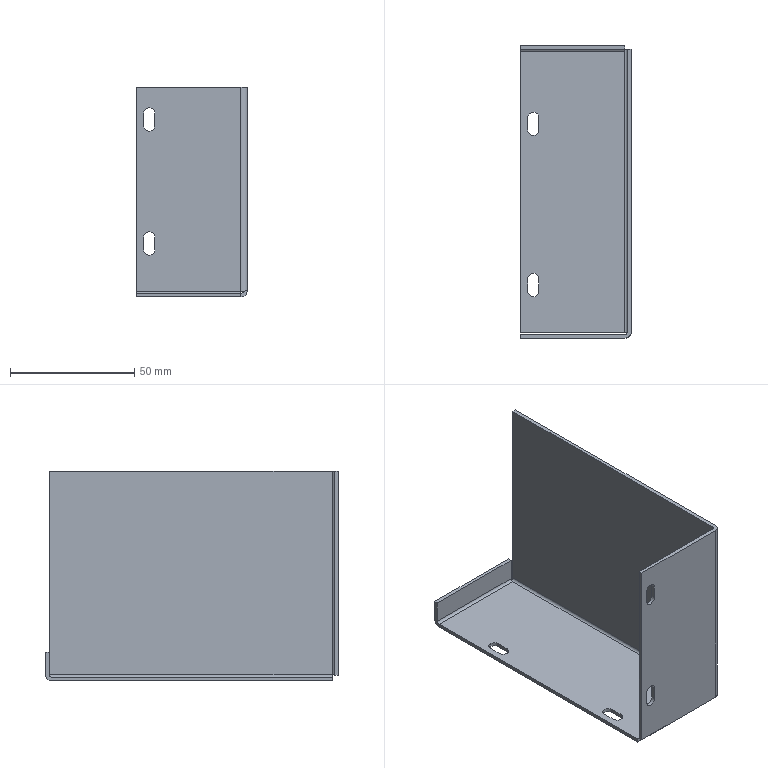Part | SolidWorks | features BaseBody 1 | 1 solid | 41 faces | box 44.5 x 118 x 84.5 mm | volume 27663 mm3 | plane 25 | cylinder 14 | spline 2 | commonest cylinder face diameters 4.5 x8 2 x3 5 x3
STEP:
#1=CARTESIAN_POINT('',(-44.5,115.,10.));
#2=VERTEX_POINT('',#1);
#3=CARTESIAN_POINT('',(-2.5,115.,10.));
#4=VERTEX_POINT('',#3);
#5=CARTESIAN_POINT('',(-2.5,115.,10.));
#6=DIRECTION('',(1.,0.,0.));
#7=VECTOR('',#6,1000.);
#8=LINE('',#5,#7);
#9=EDGE_CURVE('',#2,#4,#8,.T.);
#10=ORIENTED_EDGE('',*,*,#9,.T.);
#11=CARTESIAN_POINT('',(-2.5,116.5,10.));
#12=VERTEX_POINT('',#11);
#13=CARTESIAN_POINT('',(-2.5,116.5,10.));
#14=DIRECTION('',(0.,-1.,0.));
#15=VECTOR('',#14,1000.);
#16=LINE('',#13,#15);
#17=EDGE_CURVE('',#12,#4,#16,.T.);
#18=ORIENTED_EDGE('',*,*,#17,.F.);
#19=CARTESIAN_POINT('',(-44.5,116.5,10.));
#20=VERTEX_POINT('',#19);
#21=CARTESIAN_POINT('',(-2.5,116.5,10.));
#22=DIRECTION('',(1.,0.,0.));
#23=VECTOR('',#22,1000.);
#24=LINE('',#21,#23);
#25=EDGE_CURVE('',#20,#12,#24,.T.);
#26=ORIENTED_EDGE('',*,*,#25,.F.);
#27=CARTESIAN_POINT('',(-44.5,116.5,10.));
#28=DIRECTION('',(0.,-1.,0.));
#29=VECTOR('',#28,1000.);
#30=LINE('',#27,#29);
#31=EDGE_CURVE('',#20,#2,#30,.T.);
#32=ORIENTED_EDGE('',*,*,#31,.T.);
#33=EDGE_LOOP('',(#10,#18,#26,#32));
#34=FACE_OUTER_BOUND('',#33,.T.);
#35=CARTESIAN_POINT('',(-2.5,116.5,10.));
#36=DIRECTION('',(0.,0.,-1.));
#37=DIRECTION('',(0.,-1.,0.));
#38=AXIS2_PLACEMENT_3D('',#35,#36,#37);
#39=PLANE('',#38);
#40=ADVANCED_FACE('',(#34),#39,.F.);
#41=CARTESIAN_POINT('',(-44.5,115.,1.));
#42=VERTEX_POINT('',#41);
#43=CARTESIAN_POINT('',(-44.5,115.,10.));
#44=DIRECTION('',(0.,0.,1.));
#45=VECTOR('',#44,1000.);
#46=LINE('',#43,#45);
#47=EDGE_CURVE('',#42,#2,#46,.T.);
#48=ORIENTED_EDGE('',*,*,#47,.F.);
#49=CARTESIAN_POINT('',(-2.5,115.,1.));
#50=VERTEX_POINT('',#49);
#51=CARTESIAN_POINT('',(-2.5,115.,1.));
#52=DIRECTION('',(-1.,0.,0.));
#53=VECTOR('',#52,1000.);
#54=LINE('',#51,#53);
#55=EDGE_CURVE('',#50,#42,#54,.T.);
#56=ORIENTED_EDGE('',*,*,#55,.F.);
#57=CARTESIAN_POINT('',(-2.5,115.,0.));
#58=DIRECTION('',(0.,0.,-1.));
#59=VECTOR('',#58,1000.);
#60=LINE('',#57,#59);
#61=EDGE_CURVE('',#4,#50,#60,.T.);
#62=ORIENTED_EDGE('',*,*,#61,.F.);
#63=ORIENTED_EDGE('',*,*,#9,.F.);
#64=EDGE_LOOP('',(#48,#56,#62,#63));
#65=FACE_OUTER_BOUND('',#64,.T.);
#66=CARTESIAN_POINT('',(0.,115.,0.));
#67=DIRECTION('',(0.,-1.,0.));
#68=DIRECTION('',(-1.,0.,0.));
#69=AXIS2_PLACEMENT_3D('',#66,#67,#68);
#70=PLANE('',#69);
#71=ADVANCED_FACE('',(#65),#70,.T.);
#72=CARTESIAN_POINT('',(-44.5,116.5,1.));
#73=VERTEX_POINT('',#72);
#74=CARTESIAN_POINT('',(-2.5,116.5,1.));
#75=VERTEX_POINT('',#74);
#76=CARTESIAN_POINT('',(0.,116.5,1.));
#77=DIRECTION('',(1.,0.,0.));
#78=VECTOR('',#77,1000.);
#79=LINE('',#76,#78);
#80=EDGE_CURVE('',#73,#75,#79,.T.);
#81=ORIENTED_EDGE('',*,*,#80,.F.);
#82=CARTESIAN_POINT('',(-44.5,116.5,10.));
#83=DIRECTION('',(0.,0.,1.));
#84=VECTOR('',#83,1000.);
#85=LINE('',#82,#84);
#86=EDGE_CURVE('',#73,#20,#85,.T.);
#87=ORIENTED_EDGE('',*,*,#86,.T.);
#88=ORIENTED_EDGE('',*,*,#25,.T.);
#89=CARTESIAN_POINT('',(-2.5,116.5,0.));
#90=DIRECTION('',(0.,0.,-1.));
#91=VECTOR('',#90,1000.);
#92=LINE('',#89,#91);
#93=EDGE_CURVE('',#12,#75,#92,.T.);
#94=ORIENTED_EDGE('',*,*,#93,.T.);
#95=EDGE_LOOP('',(#81,#87,#88,#94));
#96=FACE_OUTER_BOUND('',#95,.T.);
#97=CARTESIAN_POINT('',(0.,116.5,0.));
#98=DIRECTION('',(0.,-1.,0.));
#99=DIRECTION('',(-1.,0.,0.));
#100=AXIS2_PLACEMENT_3D('',#97,#98,#99);
#101=PLANE('',#100);
#102=ADVANCED_FACE('',(#96),#101,.F.);
#103=CARTESIAN_POINT('',(-44.5,114.,0.));
#104=VERTEX_POINT('',#103);
#105=CARTESIAN_POINT('',(-2.5,114.,0.));
#106=VERTEX_POINT('',#105);
#107=CARTESIAN_POINT('',(-44.5,114.,0.));
#108=DIRECTION('',(1.,0.,0.));
#109=VECTOR('',#108,1000.);
#110=LINE('',#107,#109);
#111=EDGE_CURVE('',#104,#106,#110,.T.);
#112=ORIENTED_EDGE('',*,*,#111,.T.);
#113=CARTESIAN_POINT('',(-2.5,114.,1.));
#114=DIRECTION('',(1.,0.,0.));
#115=DIRECTION('',(0.,0.,1.));
#116=AXIS2_PLACEMENT_3D('',#113,#114,#115);
#117=CIRCLE('',#116,1.);
#118=EDGE_CURVE('',#106,#50,#117,.T.);
#119=ORIENTED_EDGE('',*,*,#118,.T.);
#120=ORIENTED_EDGE('',*,*,#55,.T.);
#121=CARTESIAN_POINT('',(-44.5,114.,1.));
#122=DIRECTION('',(-1.,0.,0.));
#123=DIRECTION('',(0.,0.,1.));
#124=AXIS2_PLACEMENT_3D('',#121,#122,#123);
#125=CIRCLE('',#124,1.);
#126=EDGE_CURVE('',#42,#104,#125,.T.);
#127=ORIENTED_EDGE('',*,*,#126,.T.);
#128=EDGE_LOOP('',(#112,#119,#120,#127));
#129=FACE_OUTER_BOUND('',#128,.T.);
#130=CARTESIAN_POINT('',(-44.5,114.,1.));
#131=DIRECTION('',(-1.,0.,0.));
#132=DIRECTION('',(0.,1.,0.));
#133=AXIS2_PLACEMENT_3D('',#130,#131,#132);
#134=CYLINDRICAL_SURFACE('',#133,1.);
#135=ADVANCED_FACE('',(#129),#134,.F.);
#136=CARTESIAN_POINT('',(-44.5,114.,-1.5));
#137=VERTEX_POINT('',#136);
#138=CARTESIAN_POINT('',(-2.5,114.,-1.5));
#139=VERTEX_POINT('',#138);
#140=CARTESIAN_POINT('',(-44.5,114.,-1.5));
#141=DIRECTION('',(1.,0.,0.));
#142=VECTOR('',#141,1000.);
#143=LINE('',#140,#142);
#144=EDGE_CURVE('',#137,#139,#143,.T.);
#145=ORIENTED_EDGE('',*,*,#144,.F.);
#146=CARTESIAN_POINT('',(-44.5,114.,1.));
#147=DIRECTION('',(-1.,0.,0.));
#148=DIRECTION('',(0.,0.,1.));
#149=AXIS2_PLACEMENT_3D('',#146,#147,#148);
#150=CIRCLE('',#149,2.5);
#151=EDGE_CURVE('',#73,#137,#150,.T.);
#152=ORIENTED_EDGE('',*,*,#151,.F.);
#153=ORIENTED_EDGE('',*,*,#80,.T.);
#154=CARTESIAN_POINT('',(-2.5,115.,-1.291));
#155=VERTEX_POINT('',#154);
#156=CARTESIAN_POINT('',(-2.5,114.,1.));
#157=DIRECTION('',(1.,0.,0.));
#158=DIRECTION('',(0.,0.,1.));
#159=AXIS2_PLACEMENT_3D('',#156,#157,#158);
#160=CIRCLE('',#159,2.5);
#161=EDGE_CURVE('',#155,#75,#160,.T.);
#162=ORIENTED_EDGE('',*,*,#161,.F.);
#163=CARTESIAN_POINT('',(-2.5,114.,1.));
#164=DIRECTION('',(1.,0.,0.));
#165=DIRECTION('',(0.,0.,1.));
#166=AXIS2_PLACEMENT_3D('',#163,#164,#165);
#167=CIRCLE('',#166,2.5);
#168=EDGE_CURVE('',#139,#155,#167,.T.);
#169=ORIENTED_EDGE('',*,*,#168,.F.);
#170=EDGE_LOOP('',(#145,#152,#153,#162,#169));
#171=FACE_OUTER_BOUND('',#170,.T.);
#172=CARTESIAN_POINT('',(-44.5,114.,1.));
#173=DIRECTION('',(-1.,0.,0.));
#174=DIRECTION('',(0.,1.,0.));
#175=AXIS2_PLACEMENT_3D('',#172,#173,#174);
#176=CYLINDRICAL_SURFACE('',#175,2.5);
#177=ADVANCED_FACE('',(#171),#176,.T.);
#178=CARTESIAN_POINT('',(-2.5,115.,0.));
#179=VERTEX_POINT('',#178);
#180=CARTESIAN_POINT('',(-2.5,115.,0.));
#181=DIRECTION('',(0.,-1.,0.));
#182=VECTOR('',#181,1000.);
#183=LINE('',#180,#182);
#184=EDGE_CURVE('',#179,#106,#183,.T.);
#185=ORIENTED_EDGE('',*,*,#184,.F.);
#186=CARTESIAN_POINT('',(-2.5,115.,0.));
#187=DIRECTION('',(0.,0.,-1.));
#188=VECTOR('',#187,1000.);
#189=LINE('',#186,#188);
#190=EDGE_CURVE('',#179,#155,#189,.T.);
#191=ORIENTED_EDGE('',*,*,#190,.T.);
#192=ORIENTED_EDGE('',*,*,#161,.T.);
#193=ORIENTED_EDGE('',*,*,#93,.F.);
#194=ORIENTED_EDGE('',*,*,#17,.T.);
#195=ORIENTED_EDGE('',*,*,#61,.T.);
#196=ORIENTED_EDGE('',*,*,#118,.F.);
#197=EDGE_LOOP('',(#185,#191,#192,#193,#194,#195,#196));
#198=FACE_OUTER_BOUND('',#197,.T.);
#199=CARTESIAN_POINT('',(-2.5,114.,1.));
#200=DIRECTION('',(1.,0.,0.));
#201=DIRECTION('',(0.,0.,1.));
#202=AXIS2_PLACEMENT_3D('',#199,#200,#201);
#203=PLANE('',#202);
#204=ADVANCED_FACE('',(#198),#203,.T.);
#205=CARTESIAN_POINT('',(-41.75,0.,72.5));
#206=VERTEX_POINT('',#205);
#207=CARTESIAN_POINT('',(-41.75,-1.5,72.5));
#208=VERTEX_POINT('',#207);
#209=CARTESIAN_POINT('',(-41.75,115.001,72.5));
#210=DIRECTION('',(0.,-1.,0.));
#211=VECTOR('',#210,1000.);
#212=LINE('',#209,#211);
#213=EDGE_CURVE('',#206,#208,#212,.T.);
#214=ORIENTED_EDGE('',*,*,#213,.T.);
#215=CARTESIAN_POINT('',(-41.75,-1.5,67.5));
#216=VERTEX_POINT('',#215);
#217=CARTESIAN_POINT('',(-41.75,-1.5,72.5));
#218=DIRECTION('',(0.,0.,-1.));
#219=VECTOR('',#218,1000.);
#220=LINE('',#217,#219);
#221=EDGE_CURVE('',#208,#216,#220,.T.);
#222=ORIENTED_EDGE('',*,*,#221,.T.);
#223=CARTESIAN_POINT('',(-41.75,0.,67.5));
#224=VERTEX_POINT('',#223);
#225=CARTESIAN_POINT('',(-41.75,115.001,67.5));
#226=DIRECTION('',(0.,-1.,0.));
#227=VECTOR('',#226,1000.);
#228=LINE('',#225,#227);
#229=EDGE_CURVE('',#224,#216,#228,.T.);
#230=ORIENTED_EDGE('',*,*,#229,.F.);
#231=CARTESIAN_POINT('',(-41.75,0.,72.5));
#232=DIRECTION('',(0.,0.,-1.));
#233=VECTOR('',#232,1000.);
#234=LINE('',#231,#233);
#235=EDGE_CURVE('',#206,#224,#234,.T.);
#236=ORIENTED_EDGE('',*,*,#235,.F.);
#237=EDGE_LOOP('',(#214,#222,#230,#236));
#238=FACE_OUTER_BOUND('',#237,.T.);
#239=CARTESIAN_POINT('',(-41.75,115.001,72.5));
#240=DIRECTION('',(-1.,0.,0.));
#241=DIRECTION('',(0.,1.,0.));
#242=AXIS2_PLACEMENT_3D('',#239,#240,#241);
#243=PLANE('',#242);
#244=ADVANCED_FACE('',(#238),#243,.F.);
#245=ORIENTED_EDGE('',*,*,#229,.T.);
#246=CARTESIAN_POINT('',(-37.25,-1.5,67.5));
#247=VERTEX_POINT('',#246);
#248=CARTESIAN_POINT('',(-39.5,-1.5,67.5));
#249=DIRECTION('',(0.,-1.,0.));
#250=DIRECTION('',(-1.,0.,0.));
#251=AXIS2_PLACEMENT_3D('',#248,#249,#250);
#252=CIRCLE('',#251,2.25);
#253=EDGE_CURVE('',#216,#247,#252,.T.);
#254=ORIENTED_EDGE('',*,*,#253,.T.);
#255=CARTESIAN_POINT('',(-37.25,0.,67.5));
#256=VERTEX_POINT('',#255);
#257=CARTESIAN_POINT('',(-37.25,115.001,67.5));
#258=DIRECTION('',(0.,-1.,0.));
#259=VECTOR('',#258,1000.);
#260=LINE('',#257,#259);
#261=EDGE_CURVE('',#256,#247,#260,.T.);
#262=ORIENTED_EDGE('',*,*,#261,.F.);
#263=CARTESIAN_POINT('',(-39.5,0.,67.5));
#264=DIRECTION('',(0.,-1.,0.));
#265=DIRECTION('',(-1.,0.,0.));
#266=AXIS2_PLACEMENT_3D('',#263,#264,#265);
#267=CIRCLE('',#266,2.25);
#268=EDGE_CURVE('',#224,#256,#267,.T.);
#269=ORIENTED_EDGE('',*,*,#268,.F.);
#270=EDGE_LOOP('',(#245,#254,#262,#269));
#271=FACE_OUTER_BOUND('',#270,.T.);
#272=CARTESIAN_POINT('',(-39.5,115.001,67.5));
#273=DIRECTION('',(0.,-1.,0.));
#274=DIRECTION('',(1.,0.,0.));
#275=AXIS2_PLACEMENT_3D('',#272,#273,#274);
#276=CYLINDRICAL_SURFACE('',#275,2.25);
#277=ADVANCED_FACE('',(#271),#276,.F.);
#278=ORIENTED_EDGE('',*,*,#261,.T.);
#279=CARTESIAN_POINT('',(-37.25,-1.5,72.5));
#280=VERTEX_POINT('',#279);
#281=CARTESIAN_POINT('',(-37.25,-1.5,72.5));
#282=DIRECTION('',(0.,0.,1.));
#283=VECTOR('',#282,1000.);
#284=LINE('',#281,#283);
#285=EDGE_CURVE('',#247,#280,#284,.T.);
#286=ORIENTED_EDGE('',*,*,#285,.T.);
#287=CARTESIAN_POINT('',(-37.25,0.,72.5));
#288=VERTEX_POINT('',#287);
#289=CARTESIAN_POINT('',(-37.25,115.001,72.5));
#290=DIRECTION('',(0.,-1.,0.));
#291=VECTOR('',#290,1000.);
#292=LINE('',#289,#291);
#293=EDGE_CURVE('',#288,#280,#292,.T.);
#294=ORIENTED_EDGE('',*,*,#293,.F.);
#295=CARTESIAN_POINT('',(-37.25,0.,72.5));
#296=DIRECTION('',(0.,0.,1.));
#297=VECTOR('',#296,1000.);
#298=LINE('',#295,#297);
#299=EDGE_CURVE('',#256,#288,#298,.T.);
#300=ORIENTED_EDGE('',*,*,#299,.F.);
#301=EDGE_LOOP('',(#278,#286,#294,#300));
#302=FACE_OUTER_BOUND('',#301,.T.);
#303=CARTESIAN_POINT('',(-37.25,115.001,72.5));
#304=DIRECTION('',(1.,0.,0.));
#305=DIRECTION('',(0.,1.,0.));
#306=AXIS2_PLACEMENT_3D('',#303,#304,#305);
#307=PLANE('',#306);
#308=ADVANCED_FACE('',(#302),#307,.F.);
#309=ORIENTED_EDGE('',*,*,#293,.T.);
#310=CARTESIAN_POINT('',(-39.5,-1.5,72.5));
#311=DIRECTION('',(0.,-1.,0.));
#312=DIRECTION('',(-1.,0.,0.));
#313=AXIS2_PLACEMENT_3D('',#310,#311,#312);
#314=CIRCLE('',#313,2.25);
#315=EDGE_CURVE('',#280,#208,#314,.T.);
#316=ORIENTED_EDGE('',*,*,#315,.T.);
#317=ORIENTED_EDGE('',*,*,#213,.F.);
#318=CARTESIAN_POINT('',(-39.5,0.,72.5));
#319=DIRECTION('',(0.,-1.,0.));
#320=DIRECTION('',(-1.,0.,0.));
#321=AXIS2_PLACEMENT_3D('',#318,#319,#320);
#322=CIRCLE('',#321,2.25);
#323=EDGE_CURVE('',#288,#206,#322,.T.);
#324=ORIENTED_EDGE('',*,*,#323,.F.);
#325=EDGE_LOOP('',(#309,#316,#317,#324));
#326=FACE_OUTER_BOUND('',#325,.T.);
#327=CARTESIAN_POINT('',(-39.5,115.001,72.5));
#328=DIRECTION('',(0.,-1.,0.));
#329=DIRECTION('',(1.,0.,0.));
#330=AXIS2_PLACEMENT_3D('',#327,#328,#329);
#331=CYLINDRICAL_SURFACE('',#330,2.25);
#332=ADVANCED_FACE('',(#326),#331,.F.);
#333=CARTESIAN_POINT('',(-37.25,0.,17.5));
#334=VERTEX_POINT('',#333);
#335=CARTESIAN_POINT('',(-37.25,-1.5,17.5));
#336=VERTEX_POINT('',#335);
#337=CARTESIAN_POINT('',(-37.25,115.001,17.5));
#338=DIRECTION('',(0.,-1.,0.));
#339=VECTOR('',#338,1000.);
#340=LINE('',#337,#339);
#341=EDGE_CURVE('',#334,#336,#340,.T.);
#342=ORIENTED_EDGE('',*,*,#341,.T.);
#343=CARTESIAN_POINT('',(-37.25,-1.5,22.5));
#344=VERTEX_POINT('',#343);
#345=CARTESIAN_POINT('',(-37.25,-1.5,17.5));
#346=DIRECTION('',(0.,0.,1.));
#347=VECTOR('',#346,1000.);
#348=LINE('',#345,#347);
#349=EDGE_CURVE('',#336,#344,#348,.T.);
#350=ORIENTED_EDGE('',*,*,#349,.T.);
#351=CARTESIAN_POINT('',(-37.25,0.,22.5));
#352=VERTEX_POINT('',#351);
#353=CARTESIAN_POINT('',(-37.25,115.001,22.5));
#354=DIRECTION('',(0.,-1.,0.));
#355=VECTOR('',#354,1000.);
#356=LINE('',#353,#355);
#357=EDGE_CURVE('',#352,#344,#356,.T.);
#358=ORIENTED_EDGE('',*,*,#357,.F.);
#359=CARTESIAN_POINT('',(-37.25,0.,17.5));
#360=DIRECTION('',(0.,0.,1.));
#361=VECTOR('',#360,1000.);
#362=LINE('',#359,#361);
#363=EDGE_CURVE('',#334,#352,#362,.T.);
#364=ORIENTED_EDGE('',*,*,#363,.F.);
#365=EDGE_LOOP('',(#342,#350,#358,#364));
#366=FACE_OUTER_BOUND('',#365,.T.);
#367=CARTESIAN_POINT('',(-37.25,115.001,17.5));
#368=DIRECTION('',(1.,0.,0.));
#369=DIRECTION('',(0.,1.,0.));
#370=AXIS2_PLACEMENT_3D('',#367,#368,#369);
#371=PLANE('',#370);
#372=ADVANCED_FACE('',(#366),#371,.F.);
#373=ORIENTED_EDGE('',*,*,#357,.T.);
#374=CARTESIAN_POINT('',(-41.75,-1.5,22.5));
#375=VERTEX_POINT('',#374);
#376=CARTESIAN_POINT('',(-39.5,-1.5,22.5));
#377=DIRECTION('',(0.,-1.,0.));
#378=DIRECTION('',(1.,0.,0.));
#379=AXIS2_PLACEMENT_3D('',#376,#377,#378);
#380=CIRCLE('',#379,2.25);
#381=EDGE_CURVE('',#344,#375,#380,.T.);
#382=ORIENTED_EDGE('',*,*,#381,.T.);
#383=CARTESIAN_POINT('',(-41.75,0.,22.5));
#384=VERTEX_POINT('',#383);
#385=CARTESIAN_POINT('',(-41.75,115.001,22.5));
#386=DIRECTION('',(0.,-1.,0.));
#387=VECTOR('',#386,1000.);
#388=LINE('',#385,#387);
#389=EDGE_CURVE('',#384,#375,#388,.T.);
#390=ORIENTED_EDGE('',*,*,#389,.F.);
#391=CARTESIAN_POINT('',(-39.5,0.,22.5));
#392=DIRECTION('',(0.,-1.,0.));
#393=DIRECTION('',(-1.,0.,0.));
#394=AXIS2_PLACEMENT_3D('',#391,#392,#393);
#395=CIRCLE('',#394,2.25);
#396=EDGE_CURVE('',#352,#384,#395,.T.);
#397=ORIENTED_EDGE('',*,*,#396,.F.);
#398=EDGE_LOOP('',(#373,#382,#390,#397));
#399=FACE_OUTER_BOUND('',#398,.T.);
#400=CARTESIAN_POINT('',(-39.5,115.001,22.5));
#401=DIRECTION('',(0.,-1.,0.));
#402=DIRECTION('',(1.,0.,0.));
#403=AXIS2_PLACEMENT_3D('',#400,#401,#402);
#404=CYLINDRICAL_SURFACE('',#403,2.25);
#405=ADVANCED_FACE('',(#399),#404,.F.);
#406=ORIENTED_EDGE('',*,*,#389,.T.);
#407=CARTESIAN_POINT('',(-41.75,-1.5,17.5));
#408=VERTEX_POINT('',#407);
#409=CARTESIAN_POINT('',(-41.75,-1.5,17.5));
#410=DIRECTION('',(0.,0.,-1.));
#411=VECTOR('',#410,1000.);
#412=LINE('',#409,#411);
#413=EDGE_CURVE('',#375,#408,#412,.T.);
#414=ORIENTED_EDGE('',*,*,#413,.T.);
#415=CARTESIAN_POINT('',(-41.75,0.,17.5));
#416=VERTEX_POINT('',#415);
#417=CARTESIAN_POINT('',(-41.75,115.001,17.5));
#418=DIRECTION('',(0.,-1.,0.));
#419=VECTOR('',#418,1000.);
#420=LINE('',#417,#419);
#421=EDGE_CURVE('',#416,#408,#420,.T.);
#422=ORIENTED_EDGE('',*,*,#421,.F.);
#423=CARTESIAN_POINT('',(-41.75,0.,17.5));
#424=DIRECTION('',(0.,0.,-1.));
#425=VECTOR('',#424,1000.);
#426=LINE('',#423,#425);
#427=EDGE_CURVE('',#384,#416,#426,.T.);
#428=ORIENTED_EDGE('',*,*,#427,.F.);
#429=EDGE_LOOP('',(#406,#414,#422,#428));
#430=FACE_OUTER_BOUND('',#429,.T.);
#431=CARTESIAN_POINT('',(-41.75,115.001,17.5));
#432=DIRECTION('',(-1.,0.,0.));
#433=DIRECTION('',(0.,1.,0.));
#434=AXIS2_PLACEMENT_3D('',#431,#432,#433);
#435=PLANE('',#434);
#436=ADVANCED_FACE('',(#430),#435,.F.);
#437=ORIENTED_EDGE('',*,*,#421,.T.);
#438=CARTESIAN_POINT('',(-39.5,-1.5,17.5));
#439=DIRECTION('',(0.,-1.,0.));
#440=DIRECTION('',(1.,0.,0.));
#441=AXIS2_PLACEMENT_3D('',#438,#439,#440);
#442=CIRCLE('',#441,2.25);
#443=EDGE_CURVE('',#408,#336,#442,.T.);
#444=ORIENTED_EDGE('',*,*,#443,.T.);
#445=ORIENTED_EDGE('',*,*,#341,.F.);
#446=CARTESIAN_POINT('',(-39.5,0.,17.5));
#447=DIRECTION('',(0.,-1.,0.));
#448=DIRECTION('',(-1.,0.,0.));
#449=AXIS2_PLACEMENT_3D('',#446,#447,#448);
#450=CIRCLE('',#449,2.25);
#451=EDGE_CURVE('',#416,#334,#450,.T.);
#452=ORIENTED_EDGE('',*,*,#451,.F.);
#453=EDGE_LOOP('',(#437,#444,#445,#452));
#454=FACE_OUTER_BOUND('',#453,.T.);
#455=CARTESIAN_POINT('',(-39.5,115.001,17.5));
#456=DIRECTION('',(0.,-1.,0.));
#457=DIRECTION('',(1.,0.,0.));
#458=AXIS2_PLACEMENT_3D('',#455,#456,#457);
#459=CYLINDRICAL_SURFACE('',#458,2.25);
#460=ADVANCED_FACE('',(#454),#459,.F.);
#461=CARTESIAN_POINT('',(-41.75,22.5,0.));
#462=VERTEX_POINT('',#461);
#463=CARTESIAN_POINT('',(-41.75,17.5,0.));
#464=VERTEX_POINT('',#463);
#465=CARTESIAN_POINT('',(-41.75,17.5,0.));
#466=DIRECTION('',(0.,-1.,0.));
#467=VECTOR('',#466,1000.);
#468=LINE('',#465,#467);
#469=EDGE_CURVE('',#462,#464,#468,.T.);
#470=ORIENTED_EDGE('',*,*,#469,.T.);
#471=CARTESIAN_POINT('',(-41.75,17.5,-1.5));
#472=VERTEX_POINT('',#471);
#473=CARTESIAN_POINT('',(-41.75,17.5,83.001));
#474=DIRECTION('',(0.,0.,-1.));
#475=VECTOR('',#474,1000.);
#476=LINE('',#473,#475);
#477=EDGE_CURVE('',#464,#472,#476,.T.);
#478=ORIENTED_EDGE('',*,*,#477,.T.);
#479=CARTESIAN_POINT('',(-41.75,22.5,-1.5));
#480=VERTEX_POINT('',#479);
#481=CARTESIAN_POINT('',(-41.75,17.5,-1.5));
#482=DIRECTION('',(0.,1.,0.));
#483=VECTOR('',#482,1000.);
#484=LINE('',#481,#483);
#485=EDGE_CURVE('',#472,#480,#484,.T.);
#486=ORIENTED_EDGE('',*,*,#485,.T.);
#487=CARTESIAN_POINT('',(-41.75,22.5,83.001));
#488=DIRECTION('',(0.,0.,-1.));
#489=VECTOR('',#488,1000.);
#490=LINE('',#487,#489);
#491=EDGE_CURVE('',#462,#480,#490,.T.);
#492=ORIENTED_EDGE('',*,*,#491,.F.);
#493=EDGE_LOOP('',(#470,#478,#486,#492));
#494=FACE_OUTER_BOUND('',#493,.T.);
#495=CARTESIAN_POINT('',(-41.75,17.5,83.001));
#496=DIRECTION('',(-1.,0.,0.));
#497=DIRECTION('',(0.,0.,1.));
#498=AXIS2_PLACEMENT_3D('',#495,#496,#497);
#499=PLANE('',#498);
#500=ADVANCED_FACE('',(#494),#499,.F.);
#501=CARTESIAN_POINT('',(-37.25,22.5,0.));
#502=VERTEX_POINT('',#501);
#503=CARTESIAN_POINT('',(-39.5,22.5,0.));
#504=DIRECTION('',(0.,0.,1.));
#505=DIRECTION('',(-1.,0.,0.));
#506=AXIS2_PLACEMENT_3D('',#503,#504,#505);
#507=CIRCLE('',#506,2.25);
#508=EDGE_CURVE('',#502,#462,#507,.T.);
#509=ORIENTED_EDGE('',*,*,#508,.T.);
#510=ORIENTED_EDGE('',*,*,#491,.T.);
#511=CARTESIAN_POINT('',(-37.25,22.5,-1.5));
#512=VERTEX_POINT('',#511);
#513=CARTESIAN_POINT('',(-39.5,22.5,-1.5));
#514=DIRECTION('',(0.,0.,-1.));
#515=DIRECTION('',(1.,0.,0.));
#516=AXIS2_PLACEMENT_3D('',#513,#514,#515);
#517=CIRCLE('',#516,2.25);
#518=EDGE_CURVE('',#480,#512,#517,.T.);
#519=ORIENTED_EDGE('',*,*,#518,.T.);
#520=CARTESIAN_POINT('',(-37.25,22.5,83.001));
#521=DIRECTION('',(0.,0.,-1.));
#522=VECTOR('',#521,1000.);
#523=LINE('',#520,#522);
#524=EDGE_CURVE('',#502,#512,#523,.T.);
#525=ORIENTED_EDGE('',*,*,#524,.F.);
#526=EDGE_LOOP('',(#509,#510,#519,#525));
#527=FACE_OUTER_BOUND('',#526,.T.);
#528=CARTESIAN_POINT('',(-39.5,22.5,83.001));
#529=DIRECTION('',(0.,0.,-1.));
#530=DIRECTION('',(-1.,0.,0.));
#531=AXIS2_PLACEMENT_3D('',#528,#529,#530);
#532=CYLINDRICAL_SURFACE('',#531,2.25);
#533=ADVANCED_FACE('',(#527),#532,.F.);
#534=CARTESIAN_POINT('',(-37.25,17.5,0.));
#535=VERTEX_POINT('',#534);
#536=CARTESIAN_POINT('',(-37.25,17.5,0.));
#537=DIRECTION('',(0.,1.,0.));
#538=VECTOR('',#537,1000.);
#539=LINE('',#536,#538);
#540=EDGE_CURVE('',#535,#502,#539,.T.);
#541=ORIENTED_EDGE('',*,*,#540,.T.);
#542=ORIENTED_EDGE('',*,*,#524,.T.);
#543=CARTESIAN_POINT('',(-37.25,17.5,-1.5));
#544=VERTEX_POINT('',#543);
#545=CARTESIAN_POINT('',(-37.25,17.5,-1.5));
#546=DIRECTION('',(0.,-1.,0.));
#547=VECTOR('',#546,1000.);
#548=LINE('',#545,#547);
#549=EDGE_CURVE('',#512,#544,#548,.T.);
#550=ORIENTED_EDGE('',*,*,#549,.T.);
#551=CARTESIAN_POINT('',(-37.25,17.5,83.001));
#552=DIRECTION('',(0.,0.,-1.));
#553=VECTOR('',#552,1000.);
#554=LINE('',#551,#553);
#555=EDGE_CURVE('',#535,#544,#554,.T.);
#556=ORIENTED_EDGE('',*,*,#555,.F.);
#557=EDGE_LOOP('',(#541,#542,#550,#556));
#558=FACE_OUTER_BOUND('',#557,.T.);
#559=CARTESIAN_POINT('',(-37.25,17.5,83.001));
#560=DIRECTION('',(1.,0.,0.));
#561=DIRECTION('',(0.,0.,1.));
#562=AXIS2_PLACEMENT_3D('',#559,#560,#561);
#563=PLANE('',#562);
#564=ADVANCED_FACE('',(#558),#563,.F.);
#565=CARTESIAN_POINT('',(-39.5,17.5,0.));
#566=DIRECTION('',(0.,0.,1.));
#567=DIRECTION('',(-1.,0.,0.));
#568=AXIS2_PLACEMENT_3D('',#565,#566,#567);
#569=CIRCLE('',#568,2.25);
#570=EDGE_CURVE('',#464,#535,#569,.T.);
#571=ORIENTED_EDGE('',*,*,#570,.T.);
#572=ORIENTED_EDGE('',*,*,#555,.T.);
#573=CARTESIAN_POINT('',(-39.5,17.5,-1.5));
#574=DIRECTION('',(0.,0.,-1.));
#575=DIRECTION('',(1.,0.,0.));
#576=AXIS2_PLACEMENT_3D('',#573,#574,#575);
#577=CIRCLE('',#576,2.25);
#578=EDGE_CURVE('',#544,#472,#577,.T.);
#579=ORIENTED_EDGE('',*,*,#578,.T.);
#580=ORIENTED_EDGE('',*,*,#477,.F.);
#581=EDGE_LOOP('',(#571,#572,#579,#580));
#582=FACE_OUTER_BOUND('',#581,.T.);
#583=CARTESIAN_POINT('',(-39.5,17.5,83.001));
#584=DIRECTION('',(0.,0.,-1.));
#585=DIRECTION('',(-1.,0.,0.));
#586=AXIS2_PLACEMENT_3D('',#583,#584,#585);
#587=CYLINDRICAL_SURFACE('',#586,2.25);
#588=ADVANCED_FACE('',(#582),#587,.F.);
#589=CARTESIAN_POINT('',(-37.25,82.5,0.));
#590=VERTEX_POINT('',#589);
#591=CARTESIAN_POINT('',(-37.25,87.5,0.));
#592=VERTEX_POINT('',#591);
#593=CARTESIAN_POINT('',(-37.25,87.5,0.));
#594=DIRECTION('',(0.,1.,0.));
#595=VECTOR('',#594,1000.);
#596=LINE('',#593,#595);
#597=EDGE_CURVE('',#590,#592,#596,.T.);
#598=ORIENTED_EDGE('',*,*,#597,.T.);
#599=CARTESIAN_POINT('',(-37.25,87.5,-1.5));
#600=VERTEX_POINT('',#599);
#601=CARTESIAN_POINT('',(-37.25,87.5,83.001));
#602=DIRECTION('',(0.,0.,-1.));
#603=VECTOR('',#602,1000.);
#604=LINE('',#601,#603);
#605=EDGE_CURVE('',#592,#600,#604,.T.);
#606=ORIENTED_EDGE('',*,*,#605,.T.);
#607=CARTESIAN_POINT('',(-37.25,82.5,-1.5));
#608=VERTEX_POINT('',#607);
#609=CARTESIAN_POINT('',(-37.25,87.5,-1.5));
#610=DIRECTION('',(0.,-1.,0.));
#611=VECTOR('',#610,1000.);
#612=LINE('',#609,#611);
#613=EDGE_CURVE('',#600,#608,#612,.T.);
#614=ORIENTED_EDGE('',*,*,#613,.T.);
#615=CARTESIAN_POINT('',(-37.25,82.5,83.001));
#616=DIRECTION('',(0.,0.,-1.));
#617=VECTOR('',#616,1000.);
#618=LINE('',#615,#617);
#619=EDGE_CURVE('',#590,#608,#618,.T.);
#620=ORIENTED_EDGE('',*,*,#619,.F.);
#621=EDGE_LOOP('',(#598,#606,#614,#620));
#622=FACE_OUTER_BOUND('',#621,.T.);
#623=CARTESIAN_POINT('',(-37.25,87.5,83.001));
#624=DIRECTION('',(1.,0.,0.));
#625=DIRECTION('',(0.,0.,1.));
#626=AXIS2_PLACEMENT_3D('',#623,#624,#625);
#627=PLANE('',#626);
#628=ADVANCED_FACE('',(#622),#627,.F.);
#629=CARTESIAN_POINT('',(-41.75,82.5,0.));
#630=VERTEX_POINT('',#629);
#631=CARTESIAN_POINT('',(-39.5,82.5,0.));
#632=DIRECTION('',(0.,0.,1.));
#633=DIRECTION('',(-1.,0.,0.));
#634=AXIS2_PLACEMENT_3D('',#631,#632,#633);
#635=CIRCLE('',#634,2.25);
#636=EDGE_CURVE('',#630,#590,#635,.T.);
#637=ORIENTED_EDGE('',*,*,#636,.T.);
#638=ORIENTED_EDGE('',*,*,#619,.T.);
#639=CARTESIAN_POINT('',(-41.75,82.5,-1.5));
#640=VERTEX_POINT('',#639);
#641=CARTESIAN_POINT('',(-39.5,82.5,-1.5));
#642=DIRECTION('',(0.,0.,-1.));
#643=DIRECTION('',(-1.,0.,0.));
#644=AXIS2_PLACEMENT_3D('',#641,#642,#643);
#645=CIRCLE('',#644,2.25);
#646=EDGE_CURVE('',#608,#640,#645,.T.);
#647=ORIENTED_EDGE('',*,*,#646,.T.);
#648=CARTESIAN_POINT('',(-41.75,82.5,83.001));
#649=DIRECTION('',(0.,0.,-1.));
#650=VECTOR('',#649,1000.);
#651=LINE('',#648,#650);
#652=EDGE_CURVE('',#630,#640,#651,.T.);
#653=ORIENTED_EDGE('',*,*,#652,.F.);
#654=EDGE_LOOP('',(#637,#638,#647,#653));
#655=FACE_OUTER_BOUND('',#654,.T.);
#656=CARTESIAN_POINT('',(-39.5,82.5,83.001));
#657=DIRECTION('',(0.,0.,-1.));
#658=DIRECTION('',(-1.,0.,0.));
#659=AXIS2_PLACEMENT_3D('',#656,#657,#658);
#660=CYLINDRICAL_SURFACE('',#659,2.25);
#661=ADVANCED_FACE('',(#655),#660,.F.);
#662=CARTESIAN_POINT('',(-41.75,87.5,0.));
#663=VERTEX_POINT('',#662);
#664=CARTESIAN_POINT('',(-41.75,87.5,0.));
#665=DIRECTION('',(0.,-1.,0.));
#666=VECTOR('',#665,1000.);
#667=LINE('',#664,#666);
#668=EDGE_CURVE('',#663,#630,#667,.T.);
#669=ORIENTED_EDGE('',*,*,#668,.T.);
#670=ORIENTED_EDGE('',*,*,#652,.T.);
#671=CARTESIAN_POINT('',(-41.75,87.5,-1.5));
#672=VERTEX_POINT('',#671);
#673=CARTESIAN_POINT('',(-41.75,87.5,-1.5));
#674=DIRECTION('',(0.,1.,0.));
#675=VECTOR('',#674,1000.);
#676=LINE('',#673,#675);
#677=EDGE_CURVE('',#640,#672,#676,.T.);
#678=ORIENTED_EDGE('',*,*,#677,.T.);
#679=CARTESIAN_POINT('',(-41.75,87.5,83.001));
#680=DIRECTION('',(0.,0.,-1.));
#681=VECTOR('',#680,1000.);
#682=LINE('',#679,#681);
#683=EDGE_CURVE('',#663,#672,#682,.T.);
#684=ORIENTED_EDGE('',*,*,#683,.F.);
#685=EDGE_LOOP('',(#669,#670,#678,#684));
#686=FACE_OUTER_BOUND('',#685,.T.);
#687=CARTESIAN_POINT('',(-41.75,87.5,83.001));
#688=DIRECTION('',(-1.,0.,0.));
#689=DIRECTION('',(0.,0.,1.));
#690=AXIS2_PLACEMENT_3D('',#687,#688,#689);
#691=PLANE('',#690);
#692=ADVANCED_FACE('',(#686),#691,.F.);
#693=CARTESIAN_POINT('',(-39.5,87.5,0.));
#694=DIRECTION('',(0.,0.,1.));
#695=DIRECTION('',(-1.,0.,0.));
#696=AXIS2_PLACEMENT_3D('',#693,#694,#695);
#697=CIRCLE('',#696,2.25);
#698=EDGE_CURVE('',#592,#663,#697,.T.);
#699=ORIENTED_EDGE('',*,*,#698,.T.);
#700=ORIENTED_EDGE('',*,*,#683,.T.);
#701=CARTESIAN_POINT('',(-39.5,87.5,-1.5));
#702=DIRECTION('',(0.,0.,-1.));
#703=DIRECTION('',(-1.,0.,0.));
#704=AXIS2_PLACEMENT_3D('',#701,#702,#703);
#705=CIRCLE('',#704,2.25);
#706=EDGE_CURVE('',#672,#600,#705,.T.);
#707=ORIENTED_EDGE('',*,*,#706,.T.);
#708=ORIENTED_EDGE('',*,*,#605,.F.);
#709=EDGE_LOOP('',(#699,#700,#707,#708));
#710=FACE_OUTER_BOUND('',#709,.T.);
#711=CARTESIAN_POINT('',(-39.5,87.5,83.001));
#712=DIRECTION('',(0.,0.,-1.));
#713=DIRECTION('',(-1.,0.,0.));
#714=AXIS2_PLACEMENT_3D('',#711,#712,#713);
#715=CYLINDRICAL_SURFACE('',#714,2.25);
#716=ADVANCED_FACE('',(#710),#715,.F.);
#717=CARTESIAN_POINT('',(-44.5,0.,0.7071));
#718=VERTEX_POINT('',#717);
#719=CARTESIAN_POINT('',(-44.5,0.,83.));
#720=VERTEX_POINT('',#719);
#721=CARTESIAN_POINT('',(-44.5,0.,0.));
#722=DIRECTION('',(0.,0.,1.));
#723=VECTOR('',#722,1000.);
#724=LINE('',#721,#723);
#725=EDGE_CURVE('',#718,#720,#724,.T.);
#726=ORIENTED_EDGE('',*,*,#725,.F.);
#727=CARTESIAN_POINT('',(-44.5,-1.5,0.7071));
#728=VERTEX_POINT('',#727);
#729=CARTESIAN_POINT('',(-44.5,-1.5,0.7071));
#730=DIRECTION('',(0.,-1.,0.));
#731=VECTOR('',#730,1000.);
#732=LINE('',#729,#731);
#733=EDGE_CURVE('',#718,#728,#732,.T.);
#734=ORIENTED_EDGE('',*,*,#733,.T.);
#735=CARTESIAN_POINT('',(-44.5,-1.5,83.));
#736=VERTEX_POINT('',#735);
#737=CARTESIAN_POINT('',(-44.5,-1.5,0.));
#738=DIRECTION('',(0.,0.,1.));
#739=VECTOR('',#738,1000.);
#740=LINE('',#737,#739);
#741=EDGE_CURVE('',#728,#736,#740,.T.);
#742=ORIENTED_EDGE('',*,*,#741,.T.);
#743=CARTESIAN_POINT('',(-44.5,-1.5,83.));
#744=DIRECTION('',(0.,1.,0.));
#745=VECTOR('',#744,1000.);
#746=LINE('',#743,#745);
#747=EDGE_CURVE('',#736,#720,#746,.T.);
#748=ORIENTED_EDGE('',*,*,#747,.T.);
#749=EDGE_LOOP('',(#726,#734,#742,#748));
#750=FACE_OUTER_BOUND('',#749,.T.);
#751=CARTESIAN_POINT('',(-44.5,-1.5,0.));
#752=DIRECTION('',(-1.,0.,0.));
#753=DIRECTION('',(0.,1.,0.));
#754=AXIS2_PLACEMENT_3D('',#751,#752,#753);
#755=PLANE('',#754);
#756=ADVANCED_FACE('',(#750),#755,.T.);
#757=ORIENTED_EDGE('',*,*,#451,.T.);
#758=ORIENTED_EDGE('',*,*,#363,.T.);
#759=ORIENTED_EDGE('',*,*,#396,.T.);
#760=ORIENTED_EDGE('',*,*,#427,.T.);
#761=EDGE_LOOP('',(#757,#758,#759,#760));
#762=FACE_BOUND('',#761,.T.);
#763=ORIENTED_EDGE('',*,*,#323,.T.);
#764=ORIENTED_EDGE('',*,*,#235,.T.);
#765=ORIENTED_EDGE('',*,*,#268,.T.);
#766=ORIENTED_EDGE('',*,*,#299,.T.);
#767=EDGE_LOOP('',(#763,#764,#765,#766));
#768=FACE_BOUND('',#767,.T.);
#769=CARTESIAN_POINT('',(-2.5,0.,0.7071));
#770=VERTEX_POINT('',#769);
#771=CARTESIAN_POINT('',(-2.5,0.,83.));
#772=VERTEX_POINT('',#771);
#773=CARTESIAN_POINT('',(-2.5,0.,0.));
#774=DIRECTION('',(0.,0.,1.));
#775=VECTOR('',#774,1000.);
#776=LINE('',#773,#775);
#777=EDGE_CURVE('',#770,#772,#776,.T.);
#778=ORIENTED_EDGE('',*,*,#777,.F.);
#779=CARTESIAN_POINT('',(-1.5,0.,0.7071));
#780=DIRECTION('',(-1.,0.,0.));
#781=VECTOR('',#780,1000.);
#782=LINE('',#779,#781);
#783=EDGE_CURVE('',#770,#718,#782,.T.);
#784=ORIENTED_EDGE('',*,*,#783,.T.);
#785=ORIENTED_EDGE('',*,*,#725,.T.);
#786=CARTESIAN_POINT('',(-44.5,0.,83.));
#787=DIRECTION('',(1.,0.,0.));
#788=VECTOR('',#787,1000.);
#789=LINE('',#786,#788);
#790=EDGE_CURVE('',#720,#772,#789,.T.);
#791=ORIENTED_EDGE('',*,*,#790,.T.);
#792=EDGE_LOOP('',(#778,#784,#785,#791));
#793=FACE_OUTER_BOUND('',#792,.T.);
#794=CARTESIAN_POINT('',(0.,0.,0.));
#795=DIRECTION('',(0.,1.,0.));
#796=DIRECTION('',(1.,0.,0.));
#797=AXIS2_PLACEMENT_3D('',#794,#795,#796);
#798=PLANE('',#797);
#799=ADVANCED_FACE('',(#762,#768,#793),#798,.T.);
#800=ORIENTED_EDGE('',*,*,#349,.F.);
#801=ORIENTED_EDGE('',*,*,#443,.F.);
#802=ORIENTED_EDGE('',*,*,#413,.F.);
#803=ORIENTED_EDGE('',*,*,#381,.F.);
#804=EDGE_LOOP('',(#800,#801,#802,#803));
#805=FACE_BOUND('',#804,.T.);
#806=ORIENTED_EDGE('',*,*,#221,.F.);
#807=ORIENTED_EDGE('',*,*,#315,.F.);
#808=ORIENTED_EDGE('',*,*,#285,.F.);
#809=ORIENTED_EDGE('',*,*,#253,.F.);
#810=EDGE_LOOP('',(#806,#807,#808,#809));
#811=FACE_BOUND('',#810,.T.);
#812=CARTESIAN_POINT('',(-2.5,-1.5,0.7071));
#813=VERTEX_POINT('',#812);
#814=CARTESIAN_POINT('',(0.,-1.5,0.7071));
#815=DIRECTION('',(-1.,0.,0.));
#816=VECTOR('',#815,1000.);
#817=LINE('',#814,#816);
#818=EDGE_CURVE('',#813,#728,#817,.T.);
#819=ORIENTED_EDGE('',*,*,#818,.F.);
#820=CARTESIAN_POINT('',(-2.5,-1.5,83.));
#821=VERTEX_POINT('',#820);
#822=CARTESIAN_POINT('',(-2.5,-1.5,0.));
#823=DIRECTION('',(0.,0.,-1.));
#824=VECTOR('',#823,1000.);
#825=LINE('',#822,#824);
#826=EDGE_CURVE('',#821,#813,#825,.T.);
#827=ORIENTED_EDGE('',*,*,#826,.F.);
#828=CARTESIAN_POINT('',(-44.5,-1.5,83.));
#829=DIRECTION('',(1.,0.,0.));
#830=VECTOR('',#829,1000.);
#831=LINE('',#828,#830);
#832=EDGE_CURVE('',#736,#821,#831,.T.);
#833=ORIENTED_EDGE('',*,*,#832,.F.);
#834=ORIENTED_EDGE('',*,*,#741,.F.);
#835=EDGE_LOOP('',(#819,#827,#833,#834));
#836=FACE_OUTER_BOUND('',#835,.T.);
#837=CARTESIAN_POINT('',(0.,-1.5,0.));
#838=DIRECTION('',(0.,1.,0.));
#839=DIRECTION('',(1.,0.,0.));
#840=AXIS2_PLACEMENT_3D('',#837,#838,#839);
#841=PLANE('',#840);
#842=ADVANCED_FACE('',(#805,#811,#836),#841,.F.);
#843=ORIENTED_EDGE('',*,*,#733,.F.);
#844=ORIENTED_EDGE('',*,*,#783,.F.);
#845=CARTESIAN_POINT('',(-2.5,0.,0.7071));
#846=DIRECTION('',(0.,1.,0.));
#847=VECTOR('',#846,1000.);
#848=LINE('',#845,#847);
#849=EDGE_CURVE('',#813,#770,#848,.T.);
#850=ORIENTED_EDGE('',*,*,#849,.F.);
#851=ORIENTED_EDGE('',*,*,#818,.T.);
#852=EDGE_LOOP('',(#843,#844,#850,#851));
#853=FACE_OUTER_BOUND('',#852,.T.);
#854=CARTESIAN_POINT('',(-1.5,0.,0.7071));
#855=DIRECTION('',(0.,0.,-1.));
#856=DIRECTION('',(-1.,0.,0.));
#857=AXIS2_PLACEMENT_3D('',#854,#855,#856);
#858=PLANE('',#857);
#859=ADVANCED_FACE('',(#853),#858,.T.);
#860=CARTESIAN_POINT('',(-1.5,1.,83.));
#861=VERTEX_POINT('',#860);
#862=CARTESIAN_POINT('',(-1.5,1.,1.));
#863=VERTEX_POINT('',#862);
#864=CARTESIAN_POINT('',(-1.5,1.,83.));
#865=DIRECTION('',(0.,0.,-1.));
#866=VECTOR('',#865,1000.);
#867=LINE('',#864,#866);
#868=EDGE_CURVE('',#861,#863,#867,.T.);
#869=ORIENTED_EDGE('',*,*,#868,.T.);
#870=CARTESIAN_POINT('',(-1.5,1.,1.));
#871=CARTESIAN_POINT('',(-1.5,0.7382,0.9512));
#872=CARTESIAN_POINT('',(-1.608,0.478,0.9024));
#873=CARTESIAN_POINT('',(-1.978,0.1078,0.8047));
#874=CARTESIAN_POINT('',(-2.238,0.,0.7559));
#875=CARTESIAN_POINT('',(-2.5,0.,0.7071));
#876=B_SPLINE_CURVE_WITH_KNOTS('',3,(#870,#871,#872,#873,#874,#875),.UNSPECIFIED.,.F.,.F.,(4,2,4),(0.,0.5,1.),.UNSPECIFIED.);
#877=EDGE_CURVE('',#863,#770,#876,.T.);
#878=ORIENTED_EDGE('',*,*,#877,.T.);
#879=ORIENTED_EDGE('',*,*,#777,.T.);
#880=CARTESIAN_POINT('',(-2.5,1.,83.));
#881=DIRECTION('',(0.,0.,1.));
#882=DIRECTION('',(0.,-1.,0.));
#883=AXIS2_PLACEMENT_3D('',#880,#881,#882);
#884=CIRCLE('',#883,1.);
#885=EDGE_CURVE('',#772,#861,#884,.T.);
#886=ORIENTED_EDGE('',*,*,#885,.T.);
#887=EDGE_LOOP('',(#869,#878,#879,#886));
#888=FACE_OUTER_BOUND('',#887,.T.);
#889=CARTESIAN_POINT('',(-2.5,1.,83.));
#890=DIRECTION('',(0.,0.,1.));
#891=DIRECTION('',(0.,-1.,0.));
#892=AXIS2_PLACEMENT_3D('',#889,#890,#891);
#893=CYLINDRICAL_SURFACE('',#892,1.);
#894=ADVANCED_FACE('',(#888),#893,.F.);
#895=CARTESIAN_POINT('',(0.,1.,83.));
#896=VERTEX_POINT('',#895);
#897=CARTESIAN_POINT('',(0.,1.,1.));
#898=VERTEX_POINT('',#897);
#899=CARTESIAN_POINT('',(0.,1.,83.));
#900=DIRECTION('',(0.,0.,-1.));
#901=VECTOR('',#900,1000.);
#902=LINE('',#899,#901);
#903=EDGE_CURVE('',#896,#898,#902,.T.);
#904=ORIENTED_EDGE('',*,*,#903,.F.);
#905=CARTESIAN_POINT('',(-2.5,1.,83.));
#906=DIRECTION('',(0.,0.,1.));
#907=DIRECTION('',(0.,-1.,0.));
#908=AXIS2_PLACEMENT_3D('',#905,#906,#907);
#909=CIRCLE('',#908,2.5);
#910=EDGE_CURVE('',#821,#896,#909,.T.);
#911=ORIENTED_EDGE('',*,*,#910,.F.);
#912=ORIENTED_EDGE('',*,*,#826,.T.);
#913=CARTESIAN_POINT('',(0.,1.,1.));
#914=CARTESIAN_POINT('',(0.,0.6728,0.9756));
#915=CARTESIAN_POINT('',(-0.06507,0.3456,0.9512));
#916=CARTESIAN_POINT('',(-0.3155,-0.259,0.9024));
#917=CARTESIAN_POINT('',(-0.5008,-0.5364,0.878));
#918=CARTESIAN_POINT('',(-0.9636,-0.9992,0.8291));
#919=CARTESIAN_POINT('',(-1.241,-1.184,0.8047));
#920=CARTESIAN_POINT('',(-1.846,-1.435,0.7559));
#921=CARTESIAN_POINT('',(-2.173,-1.5,0.7315));
#922=CARTESIAN_POINT('',(-2.5,-1.5,0.7071));
#923=B_SPLINE_CURVE_WITH_KNOTS('',3,(#913,#914,#915,#916,#917,#918,#919,#920,#921,#922),.UNSPECIFIED.,.F.,.F.,(4,2,2,2,4),(0.,0.25,0.5,0.75,1.),.UNSPECIFIED.);
#924=EDGE_CURVE('',#898,#813,#923,.T.);
#925=ORIENTED_EDGE('',*,*,#924,.F.);
#926=EDGE_LOOP('',(#904,#911,#912,#925));
#927=FACE_OUTER_BOUND('',#926,.T.);
#928=CARTESIAN_POINT('',(-2.5,1.,83.));
#929=DIRECTION('',(0.,0.,1.));
#930=DIRECTION('',(0.,-1.,0.));
#931=AXIS2_PLACEMENT_3D('',#928,#929,#930);
#932=CYLINDRICAL_SURFACE('',#931,2.5);
#933=ADVANCED_FACE('',(#927),#932,.T.);
#934=ORIENTED_EDGE('',*,*,#849,.T.);
#935=ORIENTED_EDGE('',*,*,#877,.F.);
#936=CARTESIAN_POINT('',(-1.5,1.,1.));
#937=DIRECTION('',(1.,0.,0.));
#938=VECTOR('',#937,1000.);
#939=LINE('',#936,#938);
#940=EDGE_CURVE('',#863,#898,#939,.T.);
#941=ORIENTED_EDGE('',*,*,#940,.T.);
#942=ORIENTED_EDGE('',*,*,#924,.T.);
#943=EDGE_LOOP('',(#934,#935,#941,#942));
#944=FACE_OUTER_BOUND('',#943,.T.);
#945=CARTESIAN_POINT('',(0.015,1.,1.));
#946=CARTESIAN_POINT('',(0.015,0.6707,0.9756));
#947=CARTESIAN_POINT('',(-0.05046,0.3417,0.9512));
#948=CARTESIAN_POINT('',(-0.3024,-0.2666,0.9024));
#949=CARTESIAN_POINT('',(-0.4888,-0.5456,0.878));
#950=CARTESIAN_POINT('',(-0.9544,-1.011,0.8291));
#951=CARTESIAN_POINT('',(-1.233,-1.198,0.8047));
#952=CARTESIAN_POINT('',(-1.842,-1.45,0.7559));
#953=CARTESIAN_POINT('',(-2.171,-1.515,0.7315));
#954=CARTESIAN_POINT('',(-2.5,-1.515,0.7071));
#955=CARTESIAN_POINT('',(0.,1.,1.));
#956=CARTESIAN_POINT('',(0.,0.6727,0.9756));
#957=CARTESIAN_POINT('',(-0.06507,0.3456,0.9512));
#958=CARTESIAN_POINT('',(-0.3155,-0.259,0.9024));
#959=CARTESIAN_POINT('',(-0.5008,-0.5364,0.878));
#960=CARTESIAN_POINT('',(-0.9636,-0.9992,0.8291));
#961=CARTESIAN_POINT('',(-1.241,-1.184,0.8047));
#962=CARTESIAN_POINT('',(-1.846,-1.435,0.7559));
#963=CARTESIAN_POINT('',(-2.173,-1.5,0.7315));
#964=CARTESIAN_POINT('',(-2.5,-1.5,0.7071));
#965=CARTESIAN_POINT('',(-1.5,1.,1.));
#966=CARTESIAN_POINT('',(-1.5,0.8691,0.9756));
#967=CARTESIAN_POINT('',(-1.526,0.7383,0.9512));
#968=CARTESIAN_POINT('',(-1.626,0.4964,0.9024));
#969=CARTESIAN_POINT('',(-1.7,0.3855,0.878));
#970=CARTESIAN_POINT('',(-1.885,0.2003,0.8291));
#971=CARTESIAN_POINT('',(-1.996,0.1262,0.8047));
#972=CARTESIAN_POINT('',(-2.238,0.02603,0.7559));
#973=CARTESIAN_POINT('',(-2.369,0.,0.7315));
#974=CARTESIAN_POINT('',(-2.5,0.,0.7071));
#975=CARTESIAN_POINT('',(-1.515,1.,1.));
#976=CARTESIAN_POINT('',(-1.515,0.8711,0.9756));
#977=CARTESIAN_POINT('',(-1.541,0.7422,0.9512));
#978=CARTESIAN_POINT('',(-1.639,0.504,0.9024));
#979=CARTESIAN_POINT('',(-1.712,0.3948,0.878));
#980=CARTESIAN_POINT('',(-1.895,0.2124,0.8291));
#981=CARTESIAN_POINT('',(-2.004,0.1395,0.8047));
#982=CARTESIAN_POINT('',(-2.242,0.04078,0.7559));
#983=CARTESIAN_POINT('',(-2.371,0.01515,0.7315));
#984=CARTESIAN_POINT('',(-2.5,0.01515,0.7071));
#985=B_SPLINE_SURFACE_WITH_KNOTS('',1,3,((#945,#946,#947,#948,#949,#950,#951,#952,#953,#954),(#955,#956,#957,#958,#959,#960,#961,#962,#963,#964),(#965,#966,#967,#968,#969,#970,#971,#972,#973,#974),(#975,#976,#977,#978,#979,#980,#981,#982,#983,#984)),.UNSPECIFIED.,.F.,.F.,.F.,(2,1,1,2),(4,2,2,2,4),(-0.01,0.,1.,1.01),(0.,0.25,0.5,0.75,1.),.UNSPECIFIED.);
#986=ADVANCED_FACE('',(#944),#985,.F.);
#987=CARTESIAN_POINT('',(-2.5,0.7071,0.));
#988=VERTEX_POINT('',#987);
#989=CARTESIAN_POINT('',(-44.5,0.7071,0.));
#990=VERTEX_POINT('',#989);
#991=CARTESIAN_POINT('',(-1.5,0.7071,0.));
#992=DIRECTION('',(-1.,0.,0.));
#993=VECTOR('',#992,1000.);
#994=LINE('',#991,#993);
#995=EDGE_CURVE('',#988,#990,#994,.T.);
#996=ORIENTED_EDGE('',*,*,#995,.T.);
#997=CARTESIAN_POINT('',(-44.5,0.7071,-1.5));
#998=VERTEX_POINT('',#997);
#999=CARTESIAN_POINT('',(-44.5,0.7071,-1.5));
#1000=DIRECTION('',(0.,0.,-1.));
#1001=VECTOR('',#1000,1000.);
#1002=LINE('',#999,#1001);
#1003=EDGE_CURVE('',#990,#998,#1002,.T.);
#1004=ORIENTED_EDGE('',*,*,#1003,.T.);
#1005=CARTESIAN_POINT('',(-2.5,0.7071,-1.5));
#1006=VERTEX_POINT('',#1005);
#1007=CARTESIAN_POINT('',(0.,0.7071,-1.5));
#1008=DIRECTION('',(1.,0.,0.));
#1009=VECTOR('',#1008,1000.);
#1010=LINE('',#1007,#1009);
#1011=EDGE_CURVE('',#998,#1006,#1010,.T.);
#1012=ORIENTED_EDGE('',*,*,#1011,.T.);
#1013=CARTESIAN_POINT('',(-2.5,0.7071,0.));
#1014=DIRECTION('',(0.,0.,1.));
#1015=VECTOR('',#1014,1000.);
#1016=LINE('',#1013,#1015);
#1017=EDGE_CURVE('',#1006,#988,#1016,.T.);
#1018=ORIENTED_EDGE('',*,*,#1017,.T.);
#1019=EDGE_LOOP('',(#996,#1004,#1012,#1018));
#1020=FACE_OUTER_BOUND('',#1019,.T.);
#1021=CARTESIAN_POINT('',(-1.5,0.7071,0.));
#1022=DIRECTION('',(0.,1.,0.));
#1023=DIRECTION('',(1.,0.,0.));
#1024=AXIS2_PLACEMENT_3D('',#1021,#1022,#1023);
#1025=PLANE('',#1024);
#1026=ADVANCED_FACE('',(#1020),#1025,.F.);
#1027=CARTESIAN_POINT('',(-1.5,115.,1.));
#1028=VERTEX_POINT('',#1027);
#1029=CARTESIAN_POINT('',(-1.5,0.7071,1.));
#1030=DIRECTION('',(0.,1.,0.));
#1031=VECTOR('',#1030,1000.);
#1032=LINE('',#1029,#1031);
#1033=EDGE_CURVE('',#863,#1028,#1032,.T.);
#1034=ORIENTED_EDGE('',*,*,#1033,.T.);
#1035=CARTESIAN_POINT('',(-2.5,115.,1.));
#1036=DIRECTION('',(0.,1.,0.));
#1037=DIRECTION('',(0.,0.,-1.));
#1038=AXIS2_PLACEMENT_3D('',#1035,#1036,#1037);
#1039=CIRCLE('',#1038,1.);
#1040=EDGE_CURVE('',#1028,#179,#1039,.T.);
#1041=ORIENTED_EDGE('',*,*,#1040,.T.);
#1042=ORIENTED_EDGE('',*,*,#184,.T.);
#1043=CARTESIAN_POINT('',(-2.5,115.,0.));
#1044=DIRECTION('',(0.,-1.,0.));
#1045=VECTOR('',#1044,1000.);
#1046=LINE('',#1043,#1045);
#1047=EDGE_CURVE('',#106,#988,#1046,.T.);
#1048=ORIENTED_EDGE('',*,*,#1047,.T.);
#1049=CARTESIAN_POINT('',(-2.5,0.7071,0.));
#1050=CARTESIAN_POINT('',(-2.238,0.7559,0.));
#1051=CARTESIAN_POINT('',(-1.978,0.8047,0.1078));
#1052=CARTESIAN_POINT('',(-1.608,0.9024,0.478));
#1053=CARTESIAN_POINT('',(-1.5,0.9512,0.7382));
#1054=CARTESIAN_POINT('',(-1.5,1.,1.));
#1055=B_SPLINE_CURVE_WITH_KNOTS('',3,(#1049,#1050,#1051,#1052,#1053,#1054),.UNSPECIFIED.,.F.,.F.,(4,2,4),(0.,0.5,1.),.UNSPECIFIED.);
#1056=EDGE_CURVE('',#988,#863,#1055,.T.);
#1057=ORIENTED_EDGE('',*,*,#1056,.T.);
#1058=EDGE_LOOP('',(#1034,#1041,#1042,#1048,#1057));
#1059=FACE_OUTER_BOUND('',#1058,.T.);
#1060=CARTESIAN_POINT('',(-2.5,0.7071,1.));
#1061=DIRECTION('',(0.,-1.,0.));
#1062=DIRECTION('',(0.,0.,-1.));
#1063=AXIS2_PLACEMENT_3D('',#1060,#1061,#1062);
#1064=CYLINDRICAL_SURFACE('',#1063,1.);
#1065=ADVANCED_FACE('',(#1059),#1064,.F.);
#1066=CARTESIAN_POINT('',(0.,115.,1.));
#1067=VERTEX_POINT('',#1066);
#1068=CARTESIAN_POINT('',(0.,0.7071,1.));
#1069=DIRECTION('',(0.,1.,0.));
#1070=VECTOR('',#1069,1000.);
#1071=LINE('',#1068,#1070);
#1072=EDGE_CURVE('',#898,#1067,#1071,.T.);
#1073=ORIENTED_EDGE('',*,*,#1072,.F.);
#1074=CARTESIAN_POINT('',(-2.5,0.7071,-1.5));
#1075=CARTESIAN_POINT('',(-2.173,0.7315,-1.5));
#1076=CARTESIAN_POINT('',(-1.846,0.7559,-1.435));
#1077=CARTESIAN_POINT('',(-1.241,0.8047,-1.184));
#1078=CARTESIAN_POINT('',(-0.9636,0.8291,-0.9992));
#1079=CARTESIAN_POINT('',(-0.5008,0.878,-0.5364));
#1080=CARTESIAN_POINT('',(-0.3155,0.9024,-0.259));
#1081=CARTESIAN_POINT('',(-0.06507,0.9512,0.3456));
#1082=CARTESIAN_POINT('',(0.,0.9756,0.6728));
#1083=CARTESIAN_POINT('',(0.,1.,1.));
#1084=B_SPLINE_CURVE_WITH_KNOTS('',3,(#1074,#1075,#1076,#1077,#1078,#1079,#1080,#1081,#1082,#1083),.UNSPECIFIED.,.F.,.F.,(4,2,2,2,4),(0.,0.25,0.5,0.75,1.),.UNSPECIFIED.);
#1085=EDGE_CURVE('',#1006,#898,#1084,.T.);
#1086=ORIENTED_EDGE('',*,*,#1085,.F.);
#1087=CARTESIAN_POINT('',(-2.5,0.,-1.5));
#1088=DIRECTION('',(0.,-1.,0.));
#1089=VECTOR('',#1088,1000.);
#1090=LINE('',#1087,#1089);
#1091=EDGE_CURVE('',#139,#1006,#1090,.T.);
#1092=ORIENTED_EDGE('',*,*,#1091,.F.);
#1093=CARTESIAN_POINT('',(-2.5,115.,-1.5));
#1094=VERTEX_POINT('',#1093);
#1095=CARTESIAN_POINT('',(-2.5,0.,-1.5));
#1096=DIRECTION('',(0.,-1.,0.));
#1097=VECTOR('',#1096,1000.);
#1098=LINE('',#1095,#1097);
#1099=EDGE_CURVE('',#1094,#139,#1098,.T.);
#1100=ORIENTED_EDGE('',*,*,#1099,.F.);
#1101=CARTESIAN_POINT('',(-2.5,115.,1.));
#1102=DIRECTION('',(0.,1.,0.));
#1103=DIRECTION('',(0.,0.,-1.));
#1104=AXIS2_PLACEMENT_3D('',#1101,#1102,#1103);
#1105=CIRCLE('',#1104,2.5);
#1106=EDGE_CURVE('',#1067,#1094,#1105,.T.);
#1107=ORIENTED_EDGE('',*,*,#1106,.F.);
#1108=EDGE_LOOP('',(#1073,#1086,#1092,#1100,#1107));
#1109=FACE_OUTER_BOUND('',#1108,.T.);
#1110=CARTESIAN_POINT('',(-2.5,0.7071,1.));
#1111=DIRECTION('',(0.,-1.,0.));
#1112=DIRECTION('',(0.,0.,-1.));
#1113=AXIS2_PLACEMENT_3D('',#1110,#1111,#1112);
#1114=CYLINDRICAL_SURFACE('',#1113,2.5);
#1115=ADVANCED_FACE('',(#1109),#1114,.T.);
#1116=ORIENTED_EDGE('',*,*,#1056,.F.);
#1117=ORIENTED_EDGE('',*,*,#1017,.F.);
#1118=ORIENTED_EDGE('',*,*,#1085,.T.);
#1119=ORIENTED_EDGE('',*,*,#940,.F.);
#1120=EDGE_LOOP('',(#1116,#1117,#1118,#1119));
#1121=FACE_OUTER_BOUND('',#1120,.T.);
#1122=CARTESIAN_POINT('',(-2.5,0.7071,-1.515));
#1123=CARTESIAN_POINT('',(-2.171,0.7315,-1.515));
#1124=CARTESIAN_POINT('',(-1.842,0.7559,-1.45));
#1125=CARTESIAN_POINT('',(-1.233,0.8047,-1.198));
#1126=CARTESIAN_POINT('',(-0.9544,0.8291,-1.011));
#1127=CARTESIAN_POINT('',(-0.4888,0.878,-0.5456));
#1128=CARTESIAN_POINT('',(-0.3024,0.9024,-0.2666));
#1129=CARTESIAN_POINT('',(-0.05046,0.9512,0.3417));
#1130=CARTESIAN_POINT('',(0.015,0.9756,0.6707));
#1131=CARTESIAN_POINT('',(0.015,1.,1.));
#1132=CARTESIAN_POINT('',(-2.5,0.7071,-1.5));
#1133=CARTESIAN_POINT('',(-2.173,0.7315,-1.5));
#1134=CARTESIAN_POINT('',(-1.846,0.7559,-1.435));
#1135=CARTESIAN_POINT('',(-1.241,0.8047,-1.184));
#1136=CARTESIAN_POINT('',(-0.9636,0.8291,-0.9992));
#1137=CARTESIAN_POINT('',(-0.5008,0.878,-0.5364));
#1138=CARTESIAN_POINT('',(-0.3155,0.9024,-0.259));
#1139=CARTESIAN_POINT('',(-0.06507,0.9512,0.3456));
#1140=CARTESIAN_POINT('',(0.,0.9756,0.6727));
#1141=CARTESIAN_POINT('',(0.,1.,1.));
#1142=CARTESIAN_POINT('',(-2.5,0.7071,0.));
#1143=CARTESIAN_POINT('',(-2.369,0.7315,0.));
#1144=CARTESIAN_POINT('',(-2.238,0.7559,0.02603));
#1145=CARTESIAN_POINT('',(-1.996,0.8047,0.1262));
#1146=CARTESIAN_POINT('',(-1.885,0.8291,0.2003));
#1147=CARTESIAN_POINT('',(-1.7,0.878,0.3855));
#1148=CARTESIAN_POINT('',(-1.626,0.9024,0.4964));
#1149=CARTESIAN_POINT('',(-1.526,0.9512,0.7383));
#1150=CARTESIAN_POINT('',(-1.5,0.9756,0.8691));
#1151=CARTESIAN_POINT('',(-1.5,1.,1.));
#1152=CARTESIAN_POINT('',(-2.5,0.7071,0.01515));
#1153=CARTESIAN_POINT('',(-2.371,0.7315,0.01515));
#1154=CARTESIAN_POINT('',(-2.242,0.7559,0.04078));
#1155=CARTESIAN_POINT('',(-2.004,0.8047,0.1395));
#1156=CARTESIAN_POINT('',(-1.895,0.8291,0.2124));
#1157=CARTESIAN_POINT('',(-1.712,0.878,0.3948));
#1158=CARTESIAN_POINT('',(-1.639,0.9024,0.504));
#1159=CARTESIAN_POINT('',(-1.541,0.9512,0.7422));
#1160=CARTESIAN_POINT('',(-1.515,0.9756,0.8711));
#1161=CARTESIAN_POINT('',(-1.515,1.,1.));
#1162=B_SPLINE_SURFACE_WITH_KNOTS('',1,3,((#1122,#1123,#1124,#1125,#1126,#1127,#1128,#1129,#1130,#1131),(#1132,#1133,#1134,#1135,#1136,#1137,#1138,#1139,#1140,#1141),(#1142,#1143,#1144,#1145,#1146,#1147,#1148,#1149,#1150,#1151),(#1152,#1153,#1154,#1155,#1156,#1157,#1158,#1159,#1160,#1161)),.UNSPECIFIED.,.F.,.F.,.F.,(2,1,1,2),(4,2,2,2,4),(-0.01,0.,1.,1.01),(0.,0.25,0.5,0.75,1.),.UNSPECIFIED.);
#1163=ADVANCED_FACE('',(#1121),#1162,.F.);
#1164=CARTESIAN_POINT('',(0.,115.,83.));
#1165=VERTEX_POINT('',#1164);
#1166=CARTESIAN_POINT('',(0.,115.,0.));
#1167=DIRECTION('',(0.,0.,1.));
#1168=VECTOR('',#1167,1000.);
#1169=LINE('',#1166,#1168);
#1170=EDGE_CURVE('',#1067,#1165,#1169,.T.);
#1171=ORIENTED_EDGE('',*,*,#1170,.F.);
#1172=ORIENTED_EDGE('',*,*,#1106,.T.);
#1173=CARTESIAN_POINT('',(-2.5,115.,0.));
#1174=DIRECTION('',(0.,0.,-1.));
#1175=VECTOR('',#1174,1000.);
#1176=LINE('',#1173,#1175);
#1177=EDGE_CURVE('',#155,#1094,#1176,.T.);
#1178=ORIENTED_EDGE('',*,*,#1177,.F.);
#1179=ORIENTED_EDGE('',*,*,#190,.F.);
#1180=ORIENTED_EDGE('',*,*,#1040,.F.);
#1181=CARTESIAN_POINT('',(-1.5,115.,83.));
#1182=VERTEX_POINT('',#1181);
#1183=CARTESIAN_POINT('',(-1.5,115.,0.));
#1184=DIRECTION('',(0.,0.,1.));
#1185=VECTOR('',#1184,1000.);
#1186=LINE('',#1183,#1185);
#1187=EDGE_CURVE('',#1028,#1182,#1186,.T.);
#1188=ORIENTED_EDGE('',*,*,#1187,.T.);
#1189=CARTESIAN_POINT('',(-1.5,115.,83.));
#1190=DIRECTION('',(1.,0.,0.));
#1191=VECTOR('',#1190,1000.);
#1192=LINE('',#1189,#1191);
#1193=EDGE_CURVE('',#1182,#1165,#1192,.T.);
#1194=ORIENTED_EDGE('',*,*,#1193,.T.);
#1195=EDGE_LOOP('',(#1171,#1172,#1178,#1179,#1180,#1188,#1194));
#1196=FACE_OUTER_BOUND('',#1195,.T.);
#1197=CARTESIAN_POINT('',(-1.5,115.,0.));
#1198=DIRECTION('',(0.,1.,0.));
#1199=DIRECTION('',(0.,0.,-1.));
#1200=AXIS2_PLACEMENT_3D('',#1197,#1198,#1199);
#1201=PLANE('',#1200);
#1202=ADVANCED_FACE('',(#1196),#1201,.T.);
#1203=CARTESIAN_POINT('',(-1.5,0.,83.));
#1204=DIRECTION('',(0.,-1.,0.));
#1205=VECTOR('',#1204,1000.);
#1206=LINE('',#1203,#1205);
#1207=EDGE_CURVE('',#1182,#861,#1206,.T.);
#1208=ORIENTED_EDGE('',*,*,#1207,.T.);
#1209=ORIENTED_EDGE('',*,*,#885,.F.);
#1210=ORIENTED_EDGE('',*,*,#790,.F.);
#1211=ORIENTED_EDGE('',*,*,#747,.F.);
#1212=ORIENTED_EDGE('',*,*,#832,.T.);
#1213=ORIENTED_EDGE('',*,*,#910,.T.);
#1214=CARTESIAN_POINT('',(0.,0.,83.));
#1215=DIRECTION('',(0.,-1.,0.));
#1216=VECTOR('',#1215,1000.);
#1217=LINE('',#1214,#1216);
#1218=EDGE_CURVE('',#1165,#896,#1217,.T.);
#1219=ORIENTED_EDGE('',*,*,#1218,.F.);
#1220=ORIENTED_EDGE('',*,*,#1193,.F.);
#1221=EDGE_LOOP('',(#1208,#1209,#1210,#1211,#1212,#1213,#1219,#1220));
#1222=FACE_OUTER_BOUND('',#1221,.T.);
#1223=CARTESIAN_POINT('',(-1.5,0.,83.));
#1224=DIRECTION('',(0.,0.,1.));
#1225=DIRECTION('',(1.,0.,0.));
#1226=AXIS2_PLACEMENT_3D('',#1223,#1224,#1225);
#1227=PLANE('',#1226);
#1228=ADVANCED_FACE('',(#1222),#1227,.T.);
#1229=ORIENTED_EDGE('',*,*,#1218,.T.);
#1230=ORIENTED_EDGE('',*,*,#903,.T.);
#1231=ORIENTED_EDGE('',*,*,#1072,.T.);
#1232=ORIENTED_EDGE('',*,*,#1170,.T.);
#1233=EDGE_LOOP('',(#1229,#1230,#1231,#1232));
#1234=FACE_OUTER_BOUND('',#1233,.T.);
#1235=CARTESIAN_POINT('',(0.,0.,0.));
#1236=DIRECTION('',(1.,0.,0.));
#1237=DIRECTION('',(0.,1.,0.));
#1238=AXIS2_PLACEMENT_3D('',#1235,#1236,#1237);
#1239=PLANE('',#1238);
#1240=ADVANCED_FACE('',(#1234),#1239,.T.);
#1241=ORIENTED_EDGE('',*,*,#868,.F.);
#1242=ORIENTED_EDGE('',*,*,#1207,.F.);
#1243=ORIENTED_EDGE('',*,*,#1187,.F.);
#1244=ORIENTED_EDGE('',*,*,#1033,.F.);
#1245=EDGE_LOOP('',(#1241,#1242,#1243,#1244));
#1246=FACE_OUTER_BOUND('',#1245,.T.);
#1247=CARTESIAN_POINT('',(-1.5,0.,0.));
#1248=DIRECTION('',(1.,0.,0.));
#1249=DIRECTION('',(0.,1.,0.));
#1250=AXIS2_PLACEMENT_3D('',#1247,#1248,#1249);
#1251=PLANE('',#1250);
#1252=ADVANCED_FACE('',(#1246),#1251,.F.);
#1253=CARTESIAN_POINT('',(-44.5,0.,0.));
#1254=DIRECTION('',(0.,-1.,0.));
#1255=VECTOR('',#1254,1000.);
#1256=LINE('',#1253,#1255);
#1257=EDGE_CURVE('',#104,#990,#1256,.T.);
#1258=ORIENTED_EDGE('',*,*,#1257,.F.);
#1259=ORIENTED_EDGE('',*,*,#126,.F.);
#1260=ORIENTED_EDGE('',*,*,#47,.T.);
#1261=ORIENTED_EDGE('',*,*,#31,.F.);
#1262=ORIENTED_EDGE('',*,*,#86,.F.);
#1263=ORIENTED_EDGE('',*,*,#151,.T.);
#1264=CARTESIAN_POINT('',(-44.5,0.,-1.5));
#1265=DIRECTION('',(0.,-1.,0.));
#1266=VECTOR('',#1265,1000.);
#1267=LINE('',#1264,#1266);
#1268=EDGE_CURVE('',#137,#998,#1267,.T.);
#1269=ORIENTED_EDGE('',*,*,#1268,.T.);
#1270=ORIENTED_EDGE('',*,*,#1003,.F.);
#1271=EDGE_LOOP('',(#1258,#1259,#1260,#1261,#1262,#1263,#1269,#1270));
#1272=FACE_OUTER_BOUND('',#1271,.T.);
#1273=CARTESIAN_POINT('',(-44.5,0.,-1.5));
#1274=DIRECTION('',(-1.,0.,0.));
#1275=DIRECTION('',(0.,0.,1.));
#1276=AXIS2_PLACEMENT_3D('',#1273,#1274,#1275);
#1277=PLANE('',#1276);
#1278=ADVANCED_FACE('',(#1272),#1277,.T.);
#1279=ORIENTED_EDGE('',*,*,#540,.F.);
#1280=ORIENTED_EDGE('',*,*,#570,.F.);
#1281=ORIENTED_EDGE('',*,*,#469,.F.);
#1282=ORIENTED_EDGE('',*,*,#508,.F.);
#1283=EDGE_LOOP('',(#1279,#1280,#1281,#1282));
#1284=FACE_BOUND('',#1283,.T.);
#1285=ORIENTED_EDGE('',*,*,#668,.F.);
#1286=ORIENTED_EDGE('',*,*,#698,.F.);
#1287=ORIENTED_EDGE('',*,*,#597,.F.);
#1288=ORIENTED_EDGE('',*,*,#636,.F.);
#1289=EDGE_LOOP('',(#1285,#1286,#1287,#1288));
#1290=FACE_BOUND('',#1289,.T.);
#1291=ORIENTED_EDGE('',*,*,#111,.F.);
#1292=ORIENTED_EDGE('',*,*,#1257,.T.);
#1293=ORIENTED_EDGE('',*,*,#995,.F.);
#1294=ORIENTED_EDGE('',*,*,#1047,.F.);
#1295=EDGE_LOOP('',(#1291,#1292,#1293,#1294));
#1296=FACE_OUTER_BOUND('',#1295,.T.);
#1297=CARTESIAN_POINT('',(0.,0.,0.));
#1298=DIRECTION('',(0.,0.,-1.));
#1299=DIRECTION('',(0.,-1.,0.));
#1300=AXIS2_PLACEMENT_3D('',#1297,#1298,#1299);
#1301=PLANE('',#1300);
#1302=ADVANCED_FACE('',(#1284,#1290,#1296),#1301,.F.);
#1303=ORIENTED_EDGE('',*,*,#578,.F.);
#1304=ORIENTED_EDGE('',*,*,#549,.F.);
#1305=ORIENTED_EDGE('',*,*,#518,.F.);
#1306=ORIENTED_EDGE('',*,*,#485,.F.);
#1307=EDGE_LOOP('',(#1303,#1304,#1305,#1306));
#1308=FACE_BOUND('',#1307,.T.);
#1309=ORIENTED_EDGE('',*,*,#706,.F.);
#1310=ORIENTED_EDGE('',*,*,#677,.F.);
#1311=ORIENTED_EDGE('',*,*,#646,.F.);
#1312=ORIENTED_EDGE('',*,*,#613,.F.);
#1313=EDGE_LOOP('',(#1309,#1310,#1311,#1312));
#1314=FACE_BOUND('',#1313,.T.);
#1315=ORIENTED_EDGE('',*,*,#1268,.F.);
#1316=ORIENTED_EDGE('',*,*,#144,.T.);
#1317=ORIENTED_EDGE('',*,*,#1091,.T.);
#1318=ORIENTED_EDGE('',*,*,#1011,.F.);
#1319=EDGE_LOOP('',(#1315,#1316,#1317,#1318));
#1320=FACE_OUTER_BOUND('',#1319,.T.);
#1321=CARTESIAN_POINT('',(0.,0.,-1.5));
#1322=DIRECTION('',(0.,0.,-1.));
#1323=DIRECTION('',(0.,-1.,0.));
#1324=AXIS2_PLACEMENT_3D('',#1321,#1322,#1323);
#1325=PLANE('',#1324);
#1326=ADVANCED_FACE('',(#1308,#1314,#1320),#1325,.T.);
#1327=ORIENTED_EDGE('',*,*,#1099,.T.);
#1328=ORIENTED_EDGE('',*,*,#168,.T.);
#1329=ORIENTED_EDGE('',*,*,#1177,.T.);
#1330=EDGE_LOOP('',(#1327,#1328,#1329));
#1331=FACE_OUTER_BOUND('',#1330,.T.);
#1332=CARTESIAN_POINT('',(-2.5,114.,0.));
#1333=DIRECTION('',(-1.,0.,0.));
#1334=DIRECTION('',(0.,1.,0.));
#1335=AXIS2_PLACEMENT_3D('',#1332,#1333,#1334);
#1336=PLANE('',#1335);
#1337=ADVANCED_FACE('',(#1331),#1336,.T.);
#1338=CLOSED_SHELL('',(#40,#71,#102,#135,#177,#204,#244,#277,#308,#332,#372,#405,#436,#460,#500,#533,#564,#588,#628,#661,#692,#716,#756,#799,#842,#859,#894,#933,#986,#1026,#1065,#1115,#1163,#1202,#1228,#1240,#1252,#1278,#1302,#1326,#1337));
#1339=MANIFOLD_SOLID_BREP('',#1338);
#1340=CARTESIAN_POINT('',(0.,0.,0.));
#1341=DIRECTION('',(0.,0.,1.));
#1342=DIRECTION('',(1.,0.,0.));
#1343=AXIS2_PLACEMENT_3D('',#1340,#1341,#1342);
#1344=(LENGTH_UNIT()NAMED_UNIT(*)SI_UNIT(.MILLI.,.METRE.));
#1345=UNCERTAINTY_MEASURE_WITH_UNIT(LENGTH_MEASURE(0.00001),#1344,'','');
#1346=(NAMED_UNIT(*)PLANE_ANGLE_UNIT()SI_UNIT($,.RADIAN.));
#1347=(NAMED_UNIT(*)SI_UNIT($,.STERADIAN.)SOLID_ANGLE_UNIT());
#1348=(GEOMETRIC_REPRESENTATION_CONTEXT(3)GLOBAL_UNCERTAINTY_ASSIGNED_CONTEXT((#1345))GLOBAL_UNIT_ASSIGNED_CONTEXT((#1344,#1346,#1347))REPRESENTATION_CONTEXT('',''));
#1349=ADVANCED_BREP_SHAPE_REPRESENTATION('',(#1339,#1343),#1348);